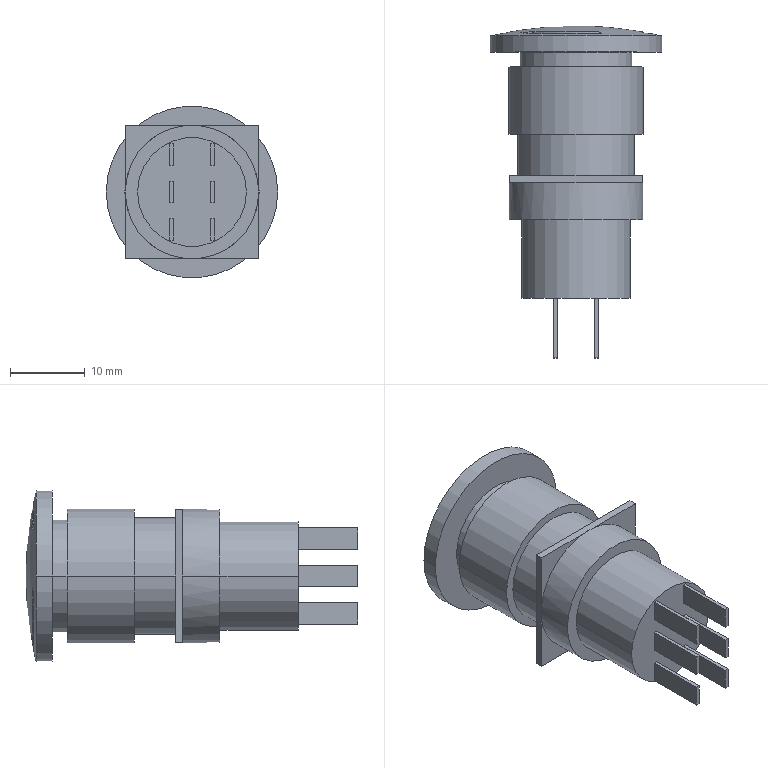Part | NX | 1 solid | 85 faces | box 23 x 44.5 x 23 mm | volume 8259 mm3 | plane 66 | cylinder 18 | sphere 1 | commonest cylinder face diameters 18 x5 20 x3 14.6 x2 15 x2 15.6 x2 17.9 x2